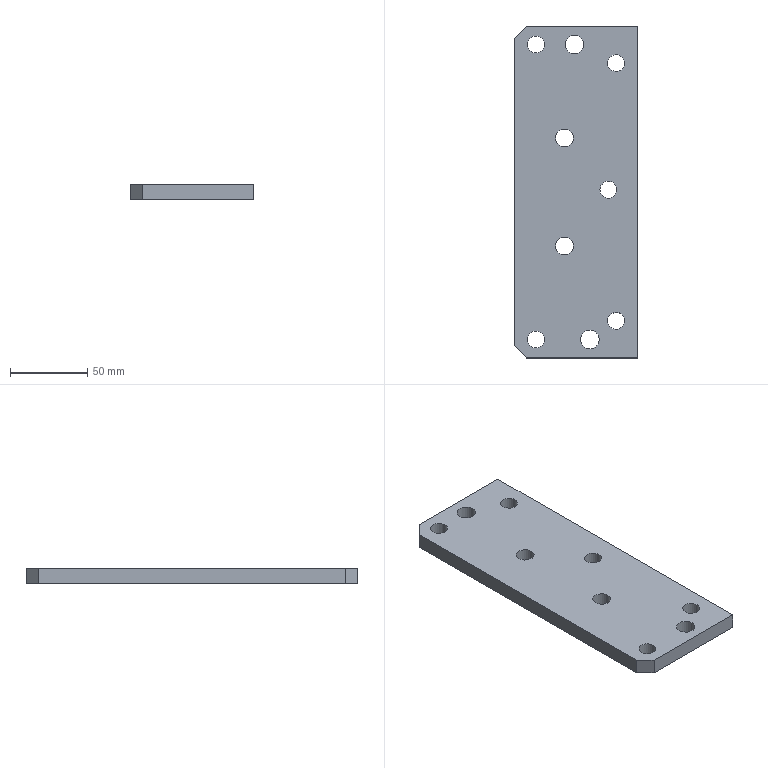Part | STEP file | lll_id2990_x_t | 1 solid | 17 faces | box 80 x 215 x 10 mm | volume 162266 mm3 | cylinder 9 | plane 8 | commonest cylinder face diameters 11 x5 11.509 x2 12 x2
STEP:
#1=CARTESIAN_POINT('',(3684.746,35.,92.5));
#2=VERTEX_POINT('',#1);
#3=CARTESIAN_POINT('',(3690.5,35.,92.5));
#4=DIRECTION('',(0.,0.,-1.));
#5=DIRECTION('',(-1.,0.,0.));
#6=AXIS2_PLACEMENT_3D('',#3,#4,#5);
#7=CIRCLE('',#6,5.755);
#8=EDGE_CURVE('',#2,#2,#7,.T.);
#9=ORIENTED_EDGE('',*,*,#8,.F.);
#10=EDGE_LOOP('',(#9));
#11=FACE_BOUND('',#10,.T.);
#12=CARTESIAN_POINT('',(3701.,-95.5,92.5));
#13=VERTEX_POINT('',#12);
#14=CARTESIAN_POINT('',(3707.,-95.5,92.5));
#15=DIRECTION('',(0.,0.,1.));
#16=DIRECTION('',(-1.,0.,0.));
#17=AXIS2_PLACEMENT_3D('',#14,#15,#16);
#18=CIRCLE('',#17,6.);
#19=EDGE_CURVE('',#13,#13,#18,.T.);
#20=ORIENTED_EDGE('',*,*,#19,.T.);
#21=EDGE_LOOP('',(#20));
#22=FACE_BOUND('',#21,.T.);
#23=CARTESIAN_POINT('',(3729.5,-83.5,92.5));
#24=VERTEX_POINT('',#23);
#25=CARTESIAN_POINT('',(3724.,-83.5,92.5));
#26=DIRECTION('',(0.,0.,1.));
#27=DIRECTION('',(1.,0.,0.));
#28=AXIS2_PLACEMENT_3D('',#25,#26,#27);
#29=CIRCLE('',#28,5.5);
#30=EDGE_CURVE('',#24,#24,#29,.T.);
#31=ORIENTED_EDGE('',*,*,#30,.T.);
#32=EDGE_LOOP('',(#31));
#33=FACE_BOUND('',#32,.T.);
#34=CARTESIAN_POINT('',(3677.5,-95.5,92.5));
#35=VERTEX_POINT('',#34);
#36=CARTESIAN_POINT('',(3672.,-95.5,92.5));
#37=DIRECTION('',(0.,0.,1.));
#38=DIRECTION('',(1.,0.,0.));
#39=AXIS2_PLACEMENT_3D('',#36,#37,#38);
#40=CIRCLE('',#39,5.5);
#41=EDGE_CURVE('',#35,#35,#40,.T.);
#42=ORIENTED_EDGE('',*,*,#41,.T.);
#43=EDGE_LOOP('',(#42));
#44=FACE_BOUND('',#43,.T.);
#45=CARTESIAN_POINT('',(3666.,-107.5,92.5));
#46=VERTEX_POINT('',#45);
#47=CARTESIAN_POINT('',(3738.,-107.5,92.5));
#48=VERTEX_POINT('',#47);
#49=CARTESIAN_POINT('',(3700.5,-107.5,92.5));
#50=DIRECTION('',(1.,0.,0.));
#51=VECTOR('',#50,1.);
#52=LINE('',#49,#51);
#53=EDGE_CURVE('',#46,#48,#52,.T.);
#54=ORIENTED_EDGE('',*,*,#53,.F.);
#55=CARTESIAN_POINT('',(3658.,-99.5,92.5));
#56=VERTEX_POINT('',#55);
#57=CARTESIAN_POINT('',(3633.5,-75.,92.5));
#58=DIRECTION('',(-0.7071,0.7071,0.));
#59=VECTOR('',#58,1.);
#60=LINE('',#57,#59);
#61=EDGE_CURVE('',#46,#56,#60,.T.);
#62=ORIENTED_EDGE('',*,*,#61,.T.);
#63=CARTESIAN_POINT('',(3658.,99.5,92.5));
#64=VERTEX_POINT('',#63);
#65=CARTESIAN_POINT('',(3658.,0.00007612,92.5));
#66=DIRECTION('',(0.,-1.,0.));
#67=VECTOR('',#66,1.);
#68=LINE('',#65,#67);
#69=EDGE_CURVE('',#64,#56,#68,.T.);
#70=ORIENTED_EDGE('',*,*,#69,.F.);
#71=CARTESIAN_POINT('',(3666.,107.5,92.5));
#72=VERTEX_POINT('',#71);
#73=CARTESIAN_POINT('',(3633.5,75.,92.5));
#74=DIRECTION('',(0.7071,0.7071,0.));
#75=VECTOR('',#74,1.);
#76=LINE('',#73,#75);
#77=EDGE_CURVE('',#64,#72,#76,.T.);
#78=ORIENTED_EDGE('',*,*,#77,.T.);
#79=CARTESIAN_POINT('',(3738.,107.5,92.5));
#80=VERTEX_POINT('',#79);
#81=CARTESIAN_POINT('',(3700.5,107.5,92.5));
#82=DIRECTION('',(-1.,0.,0.));
#83=VECTOR('',#82,1.);
#84=LINE('',#81,#83);
#85=EDGE_CURVE('',#80,#72,#84,.T.);
#86=ORIENTED_EDGE('',*,*,#85,.F.);
#87=CARTESIAN_POINT('',(3738.,0.00007612,92.5));
#88=DIRECTION('',(0.,1.,0.));
#89=VECTOR('',#88,1.);
#90=LINE('',#87,#89);
#91=EDGE_CURVE('',#48,#80,#90,.T.);
#92=ORIENTED_EDGE('',*,*,#91,.F.);
#93=EDGE_LOOP('',(#54,#62,#70,#78,#86,#92));
#94=FACE_BOUND('',#93,.T.);
#95=CARTESIAN_POINT('',(3729.5,83.5,92.5));
#96=VERTEX_POINT('',#95);
#97=CARTESIAN_POINT('',(3724.,83.5,92.5));
#98=DIRECTION('',(0.,0.,1.));
#99=DIRECTION('',(1.,0.,0.));
#100=AXIS2_PLACEMENT_3D('',#97,#98,#99);
#101=CIRCLE('',#100,5.5);
#102=EDGE_CURVE('',#96,#96,#101,.T.);
#103=ORIENTED_EDGE('',*,*,#102,.T.);
#104=EDGE_LOOP('',(#103));
#105=FACE_BOUND('',#104,.T.);
#106=CARTESIAN_POINT('',(3677.5,95.5,92.5));
#107=VERTEX_POINT('',#106);
#108=CARTESIAN_POINT('',(3672.,95.5,92.5));
#109=DIRECTION('',(0.,0.,1.));
#110=DIRECTION('',(1.,0.,0.));
#111=AXIS2_PLACEMENT_3D('',#108,#109,#110);
#112=CIRCLE('',#111,5.5);
#113=EDGE_CURVE('',#107,#107,#112,.T.);
#114=ORIENTED_EDGE('',*,*,#113,.T.);
#115=EDGE_LOOP('',(#114));
#116=FACE_BOUND('',#115,.T.);
#117=CARTESIAN_POINT('',(3691.,95.5,92.5));
#118=VERTEX_POINT('',#117);
#119=CARTESIAN_POINT('',(3697.,95.5,92.5));
#120=DIRECTION('',(0.,0.,1.));
#121=DIRECTION('',(-1.,0.,0.));
#122=AXIS2_PLACEMENT_3D('',#119,#120,#121);
#123=CIRCLE('',#122,6.);
#124=EDGE_CURVE('',#118,#118,#123,.T.);
#125=ORIENTED_EDGE('',*,*,#124,.T.);
#126=EDGE_LOOP('',(#125));
#127=FACE_BOUND('',#126,.T.);
#128=CARTESIAN_POINT('',(3713.5,1.5,92.5));
#129=VERTEX_POINT('',#128);
#130=CARTESIAN_POINT('',(3719.,1.5,92.5));
#131=DIRECTION('',(0.,0.,-1.));
#132=DIRECTION('',(-1.,0.,0.));
#133=AXIS2_PLACEMENT_3D('',#130,#131,#132);
#134=CIRCLE('',#133,5.5);
#135=EDGE_CURVE('',#129,#129,#134,.T.);
#136=ORIENTED_EDGE('',*,*,#135,.F.);
#137=EDGE_LOOP('',(#136));
#138=FACE_BOUND('',#137,.T.);
#139=CARTESIAN_POINT('',(3684.745,-35.,92.5));
#140=VERTEX_POINT('',#139);
#141=CARTESIAN_POINT('',(3690.5,-35.,92.5));
#142=DIRECTION('',(0.,0.,1.));
#143=DIRECTION('',(-1.,0.,0.));
#144=AXIS2_PLACEMENT_3D('',#141,#142,#143);
#145=CIRCLE('',#144,5.755);
#146=EDGE_CURVE('',#140,#140,#145,.T.);
#147=ORIENTED_EDGE('',*,*,#146,.T.);
#148=EDGE_LOOP('',(#147));
#149=FACE_BOUND('',#148,.T.);
#150=CARTESIAN_POINT('',(3700.5,0.00007612,92.5));
#151=DIRECTION('',(0.,0.,-1.));
#152=DIRECTION('',(1.,0.,0.));
#153=AXIS2_PLACEMENT_3D('',#150,#151,#152);
#154=PLANE('',#153);
#155=ADVANCED_FACE('',(#11,#22,#33,#44,#94,#105,#116,#127,#138,#149),#154,.T.);
#156=CARTESIAN_POINT('',(3684.746,35.,102.5));
#157=VERTEX_POINT('',#156);
#158=CARTESIAN_POINT('',(3690.5,35.,102.5));
#159=DIRECTION('',(0.,0.,-1.));
#160=DIRECTION('',(-1.,0.,0.));
#161=AXIS2_PLACEMENT_3D('',#158,#159,#160);
#162=CIRCLE('',#161,5.755);
#163=EDGE_CURVE('',#157,#157,#162,.T.);
#164=ORIENTED_EDGE('',*,*,#163,.T.);
#165=EDGE_LOOP('',(#164));
#166=FACE_BOUND('',#165,.T.);
#167=CARTESIAN_POINT('',(3718.5,83.5,102.5));
#168=VERTEX_POINT('',#167);
#169=CARTESIAN_POINT('',(3724.,83.5,102.5));
#170=DIRECTION('',(0.,0.,1.));
#171=DIRECTION('',(-1.,0.,0.));
#172=AXIS2_PLACEMENT_3D('',#169,#170,#171);
#173=CIRCLE('',#172,5.5);
#174=EDGE_CURVE('',#168,#168,#173,.T.);
#175=ORIENTED_EDGE('',*,*,#174,.F.);
#176=EDGE_LOOP('',(#175));
#177=FACE_BOUND('',#176,.T.);
#178=CARTESIAN_POINT('',(3666.5,95.5,102.5));
#179=VERTEX_POINT('',#178);
#180=CARTESIAN_POINT('',(3672.,95.5,102.5));
#181=DIRECTION('',(0.,0.,1.));
#182=DIRECTION('',(-1.,0.,0.));
#183=AXIS2_PLACEMENT_3D('',#180,#181,#182);
#184=CIRCLE('',#183,5.5);
#185=EDGE_CURVE('',#179,#179,#184,.T.);
#186=ORIENTED_EDGE('',*,*,#185,.F.);
#187=EDGE_LOOP('',(#186));
#188=FACE_BOUND('',#187,.T.);
#189=CARTESIAN_POINT('',(3691.,95.5,102.5));
#190=VERTEX_POINT('',#189);
#191=CARTESIAN_POINT('',(3697.,95.5,102.5));
#192=DIRECTION('',(0.,0.,1.));
#193=DIRECTION('',(-1.,0.,0.));
#194=AXIS2_PLACEMENT_3D('',#191,#192,#193);
#195=CIRCLE('',#194,6.);
#196=EDGE_CURVE('',#190,#190,#195,.T.);
#197=ORIENTED_EDGE('',*,*,#196,.F.);
#198=EDGE_LOOP('',(#197));
#199=FACE_BOUND('',#198,.T.);
#200=CARTESIAN_POINT('',(3713.5,1.5,102.5));
#201=VERTEX_POINT('',#200);
#202=CARTESIAN_POINT('',(3719.,1.5,102.5));
#203=DIRECTION('',(0.,0.,-1.));
#204=DIRECTION('',(-1.,0.,0.));
#205=AXIS2_PLACEMENT_3D('',#202,#203,#204);
#206=CIRCLE('',#205,5.5);
#207=EDGE_CURVE('',#201,#201,#206,.T.);
#208=ORIENTED_EDGE('',*,*,#207,.T.);
#209=EDGE_LOOP('',(#208));
#210=FACE_BOUND('',#209,.T.);
#211=CARTESIAN_POINT('',(3738.,107.5,102.5));
#212=VERTEX_POINT('',#211);
#213=CARTESIAN_POINT('',(3738.,-107.5,102.5));
#214=VERTEX_POINT('',#213);
#215=CARTESIAN_POINT('',(3738.,0.00007612,102.5));
#216=DIRECTION('',(0.,-1.,0.));
#217=VECTOR('',#216,1.);
#218=LINE('',#215,#217);
#219=EDGE_CURVE('',#212,#214,#218,.T.);
#220=ORIENTED_EDGE('',*,*,#219,.F.);
#221=CARTESIAN_POINT('',(3666.,107.5,102.5));
#222=VERTEX_POINT('',#221);
#223=CARTESIAN_POINT('',(3700.5,107.5,102.5));
#224=DIRECTION('',(-1.,0.,0.));
#225=VECTOR('',#224,1.);
#226=LINE('',#223,#225);
#227=EDGE_CURVE('',#212,#222,#226,.T.);
#228=ORIENTED_EDGE('',*,*,#227,.T.);
#229=CARTESIAN_POINT('',(3658.,99.5,102.5));
#230=VERTEX_POINT('',#229);
#231=CARTESIAN_POINT('',(3666.,107.5,102.5));
#232=DIRECTION('',(0.7071,0.7071,0.));
#233=VECTOR('',#232,1.);
#234=LINE('',#231,#233);
#235=EDGE_CURVE('',#230,#222,#234,.T.);
#236=ORIENTED_EDGE('',*,*,#235,.F.);
#237=CARTESIAN_POINT('',(3658.,-99.5,102.5));
#238=VERTEX_POINT('',#237);
#239=CARTESIAN_POINT('',(3658.,0.00007612,102.5));
#240=DIRECTION('',(0.,1.,0.));
#241=VECTOR('',#240,1.);
#242=LINE('',#239,#241);
#243=EDGE_CURVE('',#238,#230,#242,.T.);
#244=ORIENTED_EDGE('',*,*,#243,.F.);
#245=CARTESIAN_POINT('',(3666.,-107.5,102.5));
#246=VERTEX_POINT('',#245);
#247=CARTESIAN_POINT('',(3656.,-97.5,102.5));
#248=DIRECTION('',(0.7071,-0.7071,0.));
#249=VECTOR('',#248,1.);
#250=LINE('',#247,#249);
#251=EDGE_CURVE('',#238,#246,#250,.T.);
#252=ORIENTED_EDGE('',*,*,#251,.T.);
#253=CARTESIAN_POINT('',(3700.5,-107.5,102.5));
#254=DIRECTION('',(-1.,0.,0.));
#255=VECTOR('',#254,1.);
#256=LINE('',#253,#255);
#257=EDGE_CURVE('',#214,#246,#256,.T.);
#258=ORIENTED_EDGE('',*,*,#257,.F.);
#259=EDGE_LOOP('',(#220,#228,#236,#244,#252,#258));
#260=FACE_BOUND('',#259,.T.);
#261=CARTESIAN_POINT('',(3701.,-95.5,102.5));
#262=VERTEX_POINT('',#261);
#263=CARTESIAN_POINT('',(3707.,-95.5,102.5));
#264=DIRECTION('',(0.,0.,1.));
#265=DIRECTION('',(-1.,0.,0.));
#266=AXIS2_PLACEMENT_3D('',#263,#264,#265);
#267=CIRCLE('',#266,6.);
#268=EDGE_CURVE('',#262,#262,#267,.T.);
#269=ORIENTED_EDGE('',*,*,#268,.F.);
#270=EDGE_LOOP('',(#269));
#271=FACE_BOUND('',#270,.T.);
#272=CARTESIAN_POINT('',(3718.5,-83.5,102.5));
#273=VERTEX_POINT('',#272);
#274=CARTESIAN_POINT('',(3724.,-83.5,102.5));
#275=DIRECTION('',(0.,0.,1.));
#276=DIRECTION('',(-1.,0.,0.));
#277=AXIS2_PLACEMENT_3D('',#274,#275,#276);
#278=CIRCLE('',#277,5.5);
#279=EDGE_CURVE('',#273,#273,#278,.T.);
#280=ORIENTED_EDGE('',*,*,#279,.F.);
#281=EDGE_LOOP('',(#280));
#282=FACE_BOUND('',#281,.T.);
#283=CARTESIAN_POINT('',(3666.5,-95.5,102.5));
#284=VERTEX_POINT('',#283);
#285=CARTESIAN_POINT('',(3672.,-95.5,102.5));
#286=DIRECTION('',(0.,0.,1.));
#287=DIRECTION('',(-1.,0.,0.));
#288=AXIS2_PLACEMENT_3D('',#285,#286,#287);
#289=CIRCLE('',#288,5.5);
#290=EDGE_CURVE('',#284,#284,#289,.T.);
#291=ORIENTED_EDGE('',*,*,#290,.F.);
#292=EDGE_LOOP('',(#291));
#293=FACE_BOUND('',#292,.T.);
#294=CARTESIAN_POINT('',(3684.745,-35.,102.5));
#295=VERTEX_POINT('',#294);
#296=CARTESIAN_POINT('',(3690.5,-35.,102.5));
#297=DIRECTION('',(0.,0.,1.));
#298=DIRECTION('',(-1.,0.,0.));
#299=AXIS2_PLACEMENT_3D('',#296,#297,#298);
#300=CIRCLE('',#299,5.755);
#301=EDGE_CURVE('',#295,#295,#300,.T.);
#302=ORIENTED_EDGE('',*,*,#301,.F.);
#303=EDGE_LOOP('',(#302));
#304=FACE_BOUND('',#303,.T.);
#305=CARTESIAN_POINT('',(3312.867,136.288,102.5));
#306=DIRECTION('',(0.,0.,-1.));
#307=DIRECTION('',(-1.,0.,0.));
#308=AXIS2_PLACEMENT_3D('',#305,#306,#307);
#309=PLANE('',#308);
#310=ADVANCED_FACE('',(#166,#177,#188,#199,#210,#260,#271,#282,#293,#304),#309,.F.);
#311=ORIENTED_EDGE('',*,*,#227,.F.);
#312=CARTESIAN_POINT('',(3738.,107.5,92.5));
#313=DIRECTION('',(0.,0.,1.));
#314=VECTOR('',#313,1.);
#315=LINE('',#312,#314);
#316=EDGE_CURVE('',#80,#212,#315,.T.);
#317=ORIENTED_EDGE('',*,*,#316,.F.);
#318=ORIENTED_EDGE('',*,*,#85,.T.);
#319=CARTESIAN_POINT('',(3666.,107.5,92.5));
#320=DIRECTION('',(0.,0.,1.));
#321=VECTOR('',#320,1.);
#322=LINE('',#319,#321);
#323=EDGE_CURVE('',#72,#222,#322,.T.);
#324=ORIENTED_EDGE('',*,*,#323,.T.);
#325=EDGE_LOOP('',(#311,#317,#318,#324));
#326=FACE_OUTER_BOUND('',#325,.T.);
#327=CARTESIAN_POINT('',(3700.5,107.5,92.5));
#328=DIRECTION('',(0.,1.,0.));
#329=DIRECTION('',(0.,0.,-1.));
#330=AXIS2_PLACEMENT_3D('',#327,#328,#329);
#331=PLANE('',#330);
#332=ADVANCED_FACE('',(#326),#331,.T.);
#333=ORIENTED_EDGE('',*,*,#219,.T.);
#334=CARTESIAN_POINT('',(3738.,-107.5,92.5));
#335=DIRECTION('',(0.,0.,1.));
#336=VECTOR('',#335,1.);
#337=LINE('',#334,#336);
#338=EDGE_CURVE('',#48,#214,#337,.T.);
#339=ORIENTED_EDGE('',*,*,#338,.F.);
#340=ORIENTED_EDGE('',*,*,#91,.T.);
#341=ORIENTED_EDGE('',*,*,#316,.T.);
#342=EDGE_LOOP('',(#333,#339,#340,#341));
#343=FACE_OUTER_BOUND('',#342,.T.);
#344=CARTESIAN_POINT('',(3738.,0.00007612,92.5));
#345=DIRECTION('',(1.,0.,0.));
#346=DIRECTION('',(0.,0.,1.));
#347=AXIS2_PLACEMENT_3D('',#344,#345,#346);
#348=PLANE('',#347);
#349=ADVANCED_FACE('',(#343),#348,.T.);
#350=ORIENTED_EDGE('',*,*,#257,.T.);
#351=CARTESIAN_POINT('',(3666.,-107.5,92.5));
#352=DIRECTION('',(0.,0.,-1.));
#353=VECTOR('',#352,1.);
#354=LINE('',#351,#353);
#355=EDGE_CURVE('',#246,#46,#354,.T.);
#356=ORIENTED_EDGE('',*,*,#355,.T.);
#357=ORIENTED_EDGE('',*,*,#53,.T.);
#358=ORIENTED_EDGE('',*,*,#338,.T.);
#359=EDGE_LOOP('',(#350,#356,#357,#358));
#360=FACE_OUTER_BOUND('',#359,.T.);
#361=CARTESIAN_POINT('',(3700.5,-107.5,92.5));
#362=DIRECTION('',(0.,-1.,0.));
#363=DIRECTION('',(0.,0.,1.));
#364=AXIS2_PLACEMENT_3D('',#361,#362,#363);
#365=PLANE('',#364);
#366=ADVANCED_FACE('',(#360),#365,.T.);
#367=ORIENTED_EDGE('',*,*,#243,.T.);
#368=CARTESIAN_POINT('',(3658.,99.5,92.5));
#369=DIRECTION('',(0.,0.,-1.));
#370=VECTOR('',#369,1.);
#371=LINE('',#368,#370);
#372=EDGE_CURVE('',#230,#64,#371,.T.);
#373=ORIENTED_EDGE('',*,*,#372,.T.);
#374=ORIENTED_EDGE('',*,*,#69,.T.);
#375=CARTESIAN_POINT('',(3658.,-99.5,92.5));
#376=DIRECTION('',(0.,0.,1.));
#377=VECTOR('',#376,1.);
#378=LINE('',#375,#377);
#379=EDGE_CURVE('',#56,#238,#378,.T.);
#380=ORIENTED_EDGE('',*,*,#379,.T.);
#381=EDGE_LOOP('',(#367,#373,#374,#380));
#382=FACE_OUTER_BOUND('',#381,.T.);
#383=CARTESIAN_POINT('',(3658.,0.00007612,92.5));
#384=DIRECTION('',(-1.,0.,0.));
#385=DIRECTION('',(0.,0.,-1.));
#386=AXIS2_PLACEMENT_3D('',#383,#384,#385);
#387=PLANE('',#386);
#388=ADVANCED_FACE('',(#382),#387,.T.);
#389=ORIENTED_EDGE('',*,*,#174,.T.);
#390=EDGE_LOOP('',(#389));
#391=FACE_BOUND('',#390,.T.);
#392=ORIENTED_EDGE('',*,*,#102,.F.);
#393=EDGE_LOOP('',(#392));
#394=FACE_BOUND('',#393,.T.);
#395=CARTESIAN_POINT('',(3724.,83.5,92.5));
#396=DIRECTION('',(0.,0.,1.));
#397=DIRECTION('',(-1.,0.,0.));
#398=AXIS2_PLACEMENT_3D('',#395,#396,#397);
#399=CYLINDRICAL_SURFACE('',#398,5.5);
#400=ADVANCED_FACE('',(#391,#394),#399,.F.);
#401=ORIENTED_EDGE('',*,*,#290,.T.);
#402=EDGE_LOOP('',(#401));
#403=FACE_BOUND('',#402,.T.);
#404=ORIENTED_EDGE('',*,*,#41,.F.);
#405=EDGE_LOOP('',(#404));
#406=FACE_BOUND('',#405,.T.);
#407=CARTESIAN_POINT('',(3672.,-95.5,92.5));
#408=DIRECTION('',(0.,0.,1.));
#409=DIRECTION('',(-1.,0.,0.));
#410=AXIS2_PLACEMENT_3D('',#407,#408,#409);
#411=CYLINDRICAL_SURFACE('',#410,5.5);
#412=ADVANCED_FACE('',(#403,#406),#411,.F.);
#413=ORIENTED_EDGE('',*,*,#185,.T.);
#414=EDGE_LOOP('',(#413));
#415=FACE_BOUND('',#414,.T.);
#416=ORIENTED_EDGE('',*,*,#113,.F.);
#417=EDGE_LOOP('',(#416));
#418=FACE_BOUND('',#417,.T.);
#419=CARTESIAN_POINT('',(3672.,95.5,92.5));
#420=DIRECTION('',(0.,0.,1.));
#421=DIRECTION('',(-1.,0.,0.));
#422=AXIS2_PLACEMENT_3D('',#419,#420,#421);
#423=CYLINDRICAL_SURFACE('',#422,5.5);
#424=ADVANCED_FACE('',(#415,#418),#423,.F.);
#425=ORIENTED_EDGE('',*,*,#279,.T.);
#426=EDGE_LOOP('',(#425));
#427=FACE_BOUND('',#426,.T.);
#428=ORIENTED_EDGE('',*,*,#30,.F.);
#429=EDGE_LOOP('',(#428));
#430=FACE_BOUND('',#429,.T.);
#431=CARTESIAN_POINT('',(3724.,-83.5,92.5));
#432=DIRECTION('',(0.,0.,1.));
#433=DIRECTION('',(-1.,0.,0.));
#434=AXIS2_PLACEMENT_3D('',#431,#432,#433);
#435=CYLINDRICAL_SURFACE('',#434,5.5);
#436=ADVANCED_FACE('',(#427,#430),#435,.F.);
#437=ORIENTED_EDGE('',*,*,#196,.T.);
#438=EDGE_LOOP('',(#437));
#439=FACE_BOUND('',#438,.T.);
#440=ORIENTED_EDGE('',*,*,#124,.F.);
#441=EDGE_LOOP('',(#440));
#442=FACE_BOUND('',#441,.T.);
#443=CARTESIAN_POINT('',(3697.,95.5,92.5));
#444=DIRECTION('',(0.,0.,1.));
#445=DIRECTION('',(-1.,0.,0.));
#446=AXIS2_PLACEMENT_3D('',#443,#444,#445);
#447=CYLINDRICAL_SURFACE('',#446,6.);
#448=ADVANCED_FACE('',(#439,#442),#447,.F.);
#449=ORIENTED_EDGE('',*,*,#268,.T.);
#450=EDGE_LOOP('',(#449));
#451=FACE_BOUND('',#450,.T.);
#452=ORIENTED_EDGE('',*,*,#19,.F.);
#453=EDGE_LOOP('',(#452));
#454=FACE_BOUND('',#453,.T.);
#455=CARTESIAN_POINT('',(3707.,-95.5,92.5));
#456=DIRECTION('',(0.,0.,1.));
#457=DIRECTION('',(-1.,0.,0.));
#458=AXIS2_PLACEMENT_3D('',#455,#456,#457);
#459=CYLINDRICAL_SURFACE('',#458,6.);
#460=ADVANCED_FACE('',(#451,#454),#459,.F.);
#461=ORIENTED_EDGE('',*,*,#207,.F.);
#462=EDGE_LOOP('',(#461));
#463=FACE_BOUND('',#462,.T.);
#464=ORIENTED_EDGE('',*,*,#135,.T.);
#465=EDGE_LOOP('',(#464));
#466=FACE_BOUND('',#465,.T.);
#467=CARTESIAN_POINT('',(3719.,1.5,57.5));
#468=DIRECTION('',(0.,0.,1.));
#469=DIRECTION('',(-1.,0.,0.));
#470=AXIS2_PLACEMENT_3D('',#467,#468,#469);
#471=CYLINDRICAL_SURFACE('',#470,5.5);
#472=ADVANCED_FACE('',(#463,#466),#471,.F.);
#473=ORIENTED_EDGE('',*,*,#251,.F.);
#474=ORIENTED_EDGE('',*,*,#379,.F.);
#475=ORIENTED_EDGE('',*,*,#61,.F.);
#476=ORIENTED_EDGE('',*,*,#355,.F.);
#477=EDGE_LOOP('',(#473,#474,#475,#476));
#478=FACE_OUTER_BOUND('',#477,.T.);
#479=CARTESIAN_POINT('',(3656.,-97.5,92.5));
#480=DIRECTION('',(0.7071,0.7071,0.));
#481=DIRECTION('',(0.,0.,1.));
#482=AXIS2_PLACEMENT_3D('',#479,#480,#481);
#483=PLANE('',#482);
#484=ADVANCED_FACE('',(#478),#483,.F.);
#485=ORIENTED_EDGE('',*,*,#235,.T.);
#486=ORIENTED_EDGE('',*,*,#323,.F.);
#487=ORIENTED_EDGE('',*,*,#77,.F.);
#488=ORIENTED_EDGE('',*,*,#372,.F.);
#489=EDGE_LOOP('',(#485,#486,#487,#488));
#490=FACE_OUTER_BOUND('',#489,.T.);
#491=CARTESIAN_POINT('',(3666.,107.5,92.5));
#492=DIRECTION('',(0.7071,-0.7071,0.));
#493=DIRECTION('',(0.,0.,1.));
#494=AXIS2_PLACEMENT_3D('',#491,#492,#493);
#495=PLANE('',#494);
#496=ADVANCED_FACE('',(#490),#495,.F.);
#497=ORIENTED_EDGE('',*,*,#146,.F.);
#498=EDGE_LOOP('',(#497));
#499=FACE_BOUND('',#498,.T.);
#500=ORIENTED_EDGE('',*,*,#301,.T.);
#501=EDGE_LOOP('',(#500));
#502=FACE_BOUND('',#501,.T.);
#503=CARTESIAN_POINT('',(3690.5,-35.,227.5));
#504=DIRECTION('',(0.,0.,-1.));
#505=DIRECTION('',(-1.,0.,0.));
#506=AXIS2_PLACEMENT_3D('',#503,#504,#505);
#507=CYLINDRICAL_SURFACE('',#506,5.755);
#508=ADVANCED_FACE('',(#499,#502),#507,.F.);
#509=ORIENTED_EDGE('',*,*,#8,.T.);
#510=EDGE_LOOP('',(#509));
#511=FACE_BOUND('',#510,.T.);
#512=ORIENTED_EDGE('',*,*,#163,.F.);
#513=EDGE_LOOP('',(#512));
#514=FACE_BOUND('',#513,.T.);
#515=CARTESIAN_POINT('',(3690.5,35.,227.5));
#516=DIRECTION('',(0.,0.,-1.));
#517=DIRECTION('',(-1.,0.,0.));
#518=AXIS2_PLACEMENT_3D('',#515,#516,#517);
#519=CYLINDRICAL_SURFACE('',#518,5.755);
#520=ADVANCED_FACE('',(#511,#514),#519,.F.);
#521=CLOSED_SHELL('',(#155,#310,#332,#349,#366,#388,#400,#412,#424,#436,#448,#460,#472,#484,#496,#508,#520));
#522=MANIFOLD_SOLID_BREP('',#521);
#523=(LENGTH_UNIT()NAMED_UNIT(*)SI_UNIT(.MILLI.,.METRE.));
#524=UNCERTAINTY_MEASURE_WITH_UNIT(LENGTH_MEASURE(0.00002),#523,'','');
#525=(NAMED_UNIT(*)PLANE_ANGLE_UNIT()SI_UNIT($,.RADIAN.));
#526=PLANE_ANGLE_MEASURE_WITH_UNIT(PLANE_ANGLE_MEASURE(0.01745),#525);
#527=DIMENSIONAL_EXPONENTS(0.,0.,0.,0.,0.,0.,0.);
#528=(CONVERSION_BASED_UNIT('DEGREE',#526)NAMED_UNIT(#527)PLANE_ANGLE_UNIT());
#529=(NAMED_UNIT(*)SI_UNIT($,.STERADIAN.)SOLID_ANGLE_UNIT());
#530=(GEOMETRIC_REPRESENTATION_CONTEXT(3)GLOBAL_UNCERTAINTY_ASSIGNED_CONTEXT((#524))GLOBAL_UNIT_ASSIGNED_CONTEXT((#523,#528,#529))REPRESENTATION_CONTEXT('',''));
#531=ADVANCED_BREP_SHAPE_REPRESENTATION('',(#522),#530);